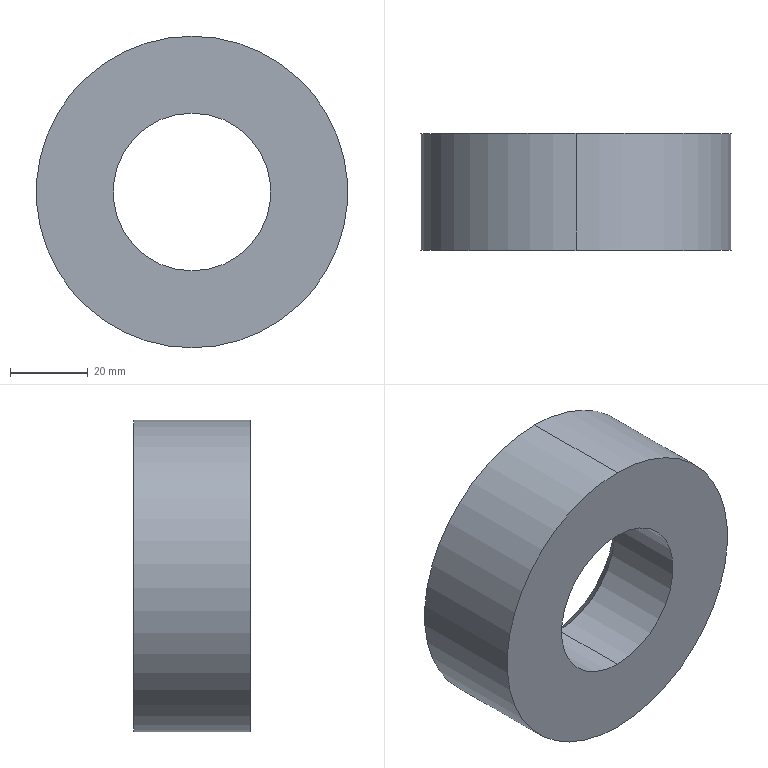Part | SolidWorks | features HoleWzd 1, Revolution 1 | 1 solid | 11 faces | box 80 x 30 x 80 mm | volume 100918 mm3 | cylinder 4 | cone 4 | plane 3 | commonest cylinder face diameters 40.5 x2 80 x2
STEP:
#1=CARTESIAN_POINT('',(0.,21.25,-20.25));
#2=VERTEX_POINT('',#1);
#3=CARTESIAN_POINT('',(0.,21.25,20.25));
#4=VERTEX_POINT('',#3);
#5=CARTESIAN_POINT('',(0.,21.25,0.));
#6=DIRECTION('',(0.,1.,0.));
#7=DIRECTION('',(0.,0.,1.));
#8=AXIS2_PLACEMENT_3D('',#5,#6,#7);
#9=CIRCLE('',#8,20.25);
#10=EDGE_CURVE('',#2,#4,#9,.T.);
#11=ORIENTED_EDGE('',*,*,#10,.T.);
#12=CARTESIAN_POINT('',(0.,0.,20.25));
#13=VERTEX_POINT('',#12);
#14=CARTESIAN_POINT('',(0.,0.,20.25));
#15=DIRECTION('',(0.,-1.,0.));
#16=VECTOR('',#15,1000.);
#17=LINE('',#14,#16);
#18=EDGE_CURVE('',#4,#13,#17,.T.);
#19=ORIENTED_EDGE('',*,*,#18,.T.);
#20=CARTESIAN_POINT('',(0.,0.,-20.25));
#21=VERTEX_POINT('',#20);
#22=CARTESIAN_POINT('',(0.,0.,0.));
#23=DIRECTION('',(0.,-1.,0.));
#24=DIRECTION('',(0.,0.,-1.));
#25=AXIS2_PLACEMENT_3D('',#22,#23,#24);
#26=CIRCLE('',#25,20.25);
#27=EDGE_CURVE('',#13,#21,#26,.T.);
#28=ORIENTED_EDGE('',*,*,#27,.T.);
#29=CARTESIAN_POINT('',(0.,0.,-20.25));
#30=DIRECTION('',(0.,-1.,0.));
#31=VECTOR('',#30,1000.);
#32=LINE('',#29,#31);
#33=EDGE_CURVE('',#2,#21,#32,.T.);
#34=ORIENTED_EDGE('',*,*,#33,.F.);
#35=EDGE_LOOP('',(#11,#19,#28,#34));
#36=FACE_OUTER_BOUND('',#35,.T.);
#37=CARTESIAN_POINT('',(0.,0.,0.));
#38=DIRECTION('',(0.,-1.,0.));
#39=DIRECTION('',(0.,0.,-1.));
#40=AXIS2_PLACEMENT_3D('',#37,#38,#39);
#41=CYLINDRICAL_SURFACE('',#40,20.25);
#42=ADVANCED_FACE('',(#36),#41,.F.);
#43=ORIENTED_EDGE('',*,*,#10,.F.);
#44=CARTESIAN_POINT('',(0.,25.,-24.));
#45=VERTEX_POINT('',#44);
#46=CARTESIAN_POINT('',(0.,25.,-24.));
#47=DIRECTION('',(0.,0.7071,-0.7071));
#48=VECTOR('',#47,1000.);
#49=LINE('',#46,#48);
#50=EDGE_CURVE('',#2,#45,#49,.T.);
#51=ORIENTED_EDGE('',*,*,#50,.T.);
#52=CARTESIAN_POINT('',(0.,25.,24.));
#53=VERTEX_POINT('',#52);
#54=CARTESIAN_POINT('',(0.,25.,0.));
#55=DIRECTION('',(0.,-1.,0.));
#56=DIRECTION('',(0.,0.,-1.));
#57=AXIS2_PLACEMENT_3D('',#54,#55,#56);
#58=CIRCLE('',#57,24.);
#59=EDGE_CURVE('',#53,#45,#58,.T.);
#60=ORIENTED_EDGE('',*,*,#59,.F.);
#61=CARTESIAN_POINT('',(0.,25.,24.));
#62=DIRECTION('',(0.,0.7071,0.7071));
#63=VECTOR('',#62,1000.);
#64=LINE('',#61,#63);
#65=EDGE_CURVE('',#4,#53,#64,.T.);
#66=ORIENTED_EDGE('',*,*,#65,.F.);
#67=EDGE_LOOP('',(#43,#51,#60,#66));
#68=FACE_OUTER_BOUND('',#67,.T.);
#69=CARTESIAN_POINT('',(0.,25.,0.));
#70=DIRECTION('',(0.,1.,0.));
#71=DIRECTION('',(0.,0.,1.));
#72=AXIS2_PLACEMENT_3D('',#69,#70,#71);
#73=CONICAL_SURFACE('',#72,24.,0.7854);
#74=ADVANCED_FACE('',(#68),#73,.F.);
#75=CARTESIAN_POINT('',(0.,25.,27.5));
#76=VERTEX_POINT('',#75);
#77=CARTESIAN_POINT('',(0.,25.,-27.5));
#78=VERTEX_POINT('',#77);
#79=CARTESIAN_POINT('',(0.,25.,0.));
#80=DIRECTION('',(0.,-1.,0.));
#81=DIRECTION('',(0.,0.,-1.));
#82=AXIS2_PLACEMENT_3D('',#79,#80,#81);
#83=CIRCLE('',#82,27.5);
#84=EDGE_CURVE('',#76,#78,#83,.T.);
#85=ORIENTED_EDGE('',*,*,#84,.T.);
#86=CARTESIAN_POINT('',(0.,30.,-37.5));
#87=VERTEX_POINT('',#86);
#88=CARTESIAN_POINT('',(0.,30.,-37.5));
#89=DIRECTION('',(0.,0.4472,-0.8944));
#90=VECTOR('',#89,1000.);
#91=LINE('',#88,#90);
#92=EDGE_CURVE('',#78,#87,#91,.T.);
#93=ORIENTED_EDGE('',*,*,#92,.T.);
#94=CARTESIAN_POINT('',(0.,30.,37.5));
#95=VERTEX_POINT('',#94);
#96=CARTESIAN_POINT('',(0.,30.,0.));
#97=DIRECTION('',(0.,-1.,0.));
#98=DIRECTION('',(0.,0.,-1.));
#99=AXIS2_PLACEMENT_3D('',#96,#97,#98);
#100=CIRCLE('',#99,37.5);
#101=EDGE_CURVE('',#95,#87,#100,.T.);
#102=ORIENTED_EDGE('',*,*,#101,.F.);
#103=CARTESIAN_POINT('',(0.,30.,37.5));
#104=DIRECTION('',(0.,0.4472,0.8944));
#105=VECTOR('',#104,1000.);
#106=LINE('',#103,#105);
#107=EDGE_CURVE('',#76,#95,#106,.T.);
#108=ORIENTED_EDGE('',*,*,#107,.F.);
#109=EDGE_LOOP('',(#85,#93,#102,#108));
#110=FACE_OUTER_BOUND('',#109,.T.);
#111=CARTESIAN_POINT('',(0.,30.,0.));
#112=DIRECTION('',(0.,1.,0.));
#113=DIRECTION('',(0.,0.,1.));
#114=AXIS2_PLACEMENT_3D('',#111,#112,#113);
#115=CONICAL_SURFACE('',#114,37.5,1.107);
#116=ADVANCED_FACE('',(#110),#115,.F.);
#117=CARTESIAN_POINT('',(0.,30.,-40.));
#118=VERTEX_POINT('',#117);
#119=CARTESIAN_POINT('',(0.,30.,40.));
#120=VERTEX_POINT('',#119);
#121=CARTESIAN_POINT('',(0.,30.,0.));
#122=DIRECTION('',(0.,-1.,0.));
#123=DIRECTION('',(0.,0.,-1.));
#124=AXIS2_PLACEMENT_3D('',#121,#122,#123);
#125=CIRCLE('',#124,40.);
#126=EDGE_CURVE('',#118,#120,#125,.T.);
#127=ORIENTED_EDGE('',*,*,#126,.T.);
#128=CARTESIAN_POINT('',(0.,0.,40.));
#129=VERTEX_POINT('',#128);
#130=CARTESIAN_POINT('',(0.,0.,40.));
#131=DIRECTION('',(0.,-1.,0.));
#132=VECTOR('',#131,1000.);
#133=LINE('',#130,#132);
#134=EDGE_CURVE('',#120,#129,#133,.T.);
#135=ORIENTED_EDGE('',*,*,#134,.T.);
#136=CARTESIAN_POINT('',(0.,0.,-40.));
#137=VERTEX_POINT('',#136);
#138=CARTESIAN_POINT('',(0.,0.,0.));
#139=DIRECTION('',(0.,-1.,0.));
#140=DIRECTION('',(0.,0.,-1.));
#141=AXIS2_PLACEMENT_3D('',#138,#139,#140);
#142=CIRCLE('',#141,40.);
#143=EDGE_CURVE('',#137,#129,#142,.T.);
#144=ORIENTED_EDGE('',*,*,#143,.F.);
#145=CARTESIAN_POINT('',(0.,0.,-40.));
#146=DIRECTION('',(0.,-1.,0.));
#147=VECTOR('',#146,1000.);
#148=LINE('',#145,#147);
#149=EDGE_CURVE('',#118,#137,#148,.T.);
#150=ORIENTED_EDGE('',*,*,#149,.F.);
#151=EDGE_LOOP('',(#127,#135,#144,#150));
#152=FACE_OUTER_BOUND('',#151,.T.);
#153=CARTESIAN_POINT('',(0.,0.,0.));
#154=DIRECTION('',(0.,-1.,0.));
#155=DIRECTION('',(0.,0.,-1.));
#156=AXIS2_PLACEMENT_3D('',#153,#154,#155);
#157=CYLINDRICAL_SURFACE('',#156,40.);
#158=ADVANCED_FACE('',(#152),#157,.T.);
#159=ORIENTED_EDGE('',*,*,#134,.F.);
#160=CARTESIAN_POINT('',(0.,30.,0.));
#161=DIRECTION('',(0.,-1.,0.));
#162=DIRECTION('',(0.,0.,-1.));
#163=AXIS2_PLACEMENT_3D('',#160,#161,#162);
#164=CIRCLE('',#163,40.);
#165=EDGE_CURVE('',#120,#118,#164,.T.);
#166=ORIENTED_EDGE('',*,*,#165,.T.);
#167=ORIENTED_EDGE('',*,*,#149,.T.);
#168=CARTESIAN_POINT('',(0.,0.,0.));
#169=DIRECTION('',(0.,-1.,0.));
#170=DIRECTION('',(0.,0.,-1.));
#171=AXIS2_PLACEMENT_3D('',#168,#169,#170);
#172=CIRCLE('',#171,40.);
#173=EDGE_CURVE('',#129,#137,#172,.T.);
#174=ORIENTED_EDGE('',*,*,#173,.F.);
#175=EDGE_LOOP('',(#159,#166,#167,#174));
#176=FACE_OUTER_BOUND('',#175,.T.);
#177=CARTESIAN_POINT('',(0.,0.,0.));
#178=DIRECTION('',(0.,-1.,0.));
#179=DIRECTION('',(0.,0.,-1.));
#180=AXIS2_PLACEMENT_3D('',#177,#178,#179);
#181=CYLINDRICAL_SURFACE('',#180,40.);
#182=ADVANCED_FACE('',(#176),#181,.T.);
#183=ORIENTED_EDGE('',*,*,#101,.T.);
#184=CARTESIAN_POINT('',(0.,30.,0.));
#185=DIRECTION('',(0.,-1.,0.));
#186=DIRECTION('',(0.,0.,-1.));
#187=AXIS2_PLACEMENT_3D('',#184,#185,#186);
#188=CIRCLE('',#187,37.5);
#189=EDGE_CURVE('',#87,#95,#188,.T.);
#190=ORIENTED_EDGE('',*,*,#189,.T.);
#191=EDGE_LOOP('',(#183,#190));
#192=FACE_BOUND('',#191,.T.);
#193=ORIENTED_EDGE('',*,*,#126,.F.);
#194=ORIENTED_EDGE('',*,*,#165,.F.);
#195=EDGE_LOOP('',(#193,#194));
#196=FACE_OUTER_BOUND('',#195,.T.);
#197=CARTESIAN_POINT('',(40.,30.,0.));
#198=DIRECTION('',(0.,1.,0.));
#199=DIRECTION('',(0.,0.,1.));
#200=AXIS2_PLACEMENT_3D('',#197,#198,#199);
#201=PLANE('',#200);
#202=ADVANCED_FACE('',(#192,#196),#201,.T.);
#203=ORIENTED_EDGE('',*,*,#92,.F.);
#204=CARTESIAN_POINT('',(0.,25.,0.));
#205=DIRECTION('',(0.,-1.,0.));
#206=DIRECTION('',(0.,0.,-1.));
#207=AXIS2_PLACEMENT_3D('',#204,#205,#206);
#208=CIRCLE('',#207,27.5);
#209=EDGE_CURVE('',#78,#76,#208,.T.);
#210=ORIENTED_EDGE('',*,*,#209,.T.);
#211=ORIENTED_EDGE('',*,*,#107,.T.);
#212=ORIENTED_EDGE('',*,*,#189,.F.);
#213=EDGE_LOOP('',(#203,#210,#211,#212));
#214=FACE_OUTER_BOUND('',#213,.T.);
#215=CARTESIAN_POINT('',(0.,30.,0.));
#216=DIRECTION('',(0.,1.,0.));
#217=DIRECTION('',(0.,0.,1.));
#218=AXIS2_PLACEMENT_3D('',#215,#216,#217);
#219=CONICAL_SURFACE('',#218,37.5,1.107);
#220=ADVANCED_FACE('',(#214),#219,.F.);
#221=ORIENTED_EDGE('',*,*,#59,.T.);
#222=CARTESIAN_POINT('',(0.,25.,0.));
#223=DIRECTION('',(0.,-1.,0.));
#224=DIRECTION('',(0.,0.,-1.));
#225=AXIS2_PLACEMENT_3D('',#222,#223,#224);
#226=CIRCLE('',#225,24.);
#227=EDGE_CURVE('',#45,#53,#226,.T.);
#228=ORIENTED_EDGE('',*,*,#227,.T.);
#229=EDGE_LOOP('',(#221,#228));
#230=FACE_BOUND('',#229,.T.);
#231=ORIENTED_EDGE('',*,*,#84,.F.);
#232=ORIENTED_EDGE('',*,*,#209,.F.);
#233=EDGE_LOOP('',(#231,#232));
#234=FACE_OUTER_BOUND('',#233,.T.);
#235=CARTESIAN_POINT('',(27.5,25.,0.));
#236=DIRECTION('',(0.,1.,0.));
#237=DIRECTION('',(0.,0.,1.));
#238=AXIS2_PLACEMENT_3D('',#235,#236,#237);
#239=PLANE('',#238);
#240=ADVANCED_FACE('',(#230,#234),#239,.T.);
#241=ORIENTED_EDGE('',*,*,#50,.F.);
#242=CARTESIAN_POINT('',(0.,21.25,0.));
#243=DIRECTION('',(0.,1.,0.));
#244=DIRECTION('',(0.,0.,1.));
#245=AXIS2_PLACEMENT_3D('',#242,#243,#244);
#246=CIRCLE('',#245,20.25);
#247=EDGE_CURVE('',#4,#2,#246,.T.);
#248=ORIENTED_EDGE('',*,*,#247,.F.);
#249=ORIENTED_EDGE('',*,*,#65,.T.);
#250=ORIENTED_EDGE('',*,*,#227,.F.);
#251=EDGE_LOOP('',(#241,#248,#249,#250));
#252=FACE_OUTER_BOUND('',#251,.T.);
#253=CARTESIAN_POINT('',(0.,25.,0.));
#254=DIRECTION('',(0.,1.,0.));
#255=DIRECTION('',(0.,0.,1.));
#256=AXIS2_PLACEMENT_3D('',#253,#254,#255);
#257=CONICAL_SURFACE('',#256,24.,0.7854);
#258=ADVANCED_FACE('',(#252),#257,.F.);
#259=CARTESIAN_POINT('',(0.,0.,0.));
#260=DIRECTION('',(0.,-1.,0.));
#261=DIRECTION('',(0.,0.,-1.));
#262=AXIS2_PLACEMENT_3D('',#259,#260,#261);
#263=CIRCLE('',#262,20.25);
#264=EDGE_CURVE('',#21,#13,#263,.T.);
#265=ORIENTED_EDGE('',*,*,#264,.F.);
#266=ORIENTED_EDGE('',*,*,#27,.F.);
#267=EDGE_LOOP('',(#265,#266));
#268=FACE_BOUND('',#267,.T.);
#269=ORIENTED_EDGE('',*,*,#143,.T.);
#270=ORIENTED_EDGE('',*,*,#173,.T.);
#271=EDGE_LOOP('',(#269,#270));
#272=FACE_OUTER_BOUND('',#271,.T.);
#273=CARTESIAN_POINT('',(20.,0.,0.));
#274=DIRECTION('',(0.,-1.,0.));
#275=DIRECTION('',(0.,0.,-1.));
#276=AXIS2_PLACEMENT_3D('',#273,#274,#275);
#277=PLANE('',#276);
#278=ADVANCED_FACE('',(#268,#272),#277,.T.);
#279=ORIENTED_EDGE('',*,*,#18,.F.);
#280=ORIENTED_EDGE('',*,*,#247,.T.);
#281=ORIENTED_EDGE('',*,*,#33,.T.);
#282=ORIENTED_EDGE('',*,*,#264,.T.);
#283=EDGE_LOOP('',(#279,#280,#281,#282));
#284=FACE_OUTER_BOUND('',#283,.T.);
#285=CARTESIAN_POINT('',(0.,0.,0.));
#286=DIRECTION('',(0.,-1.,0.));
#287=DIRECTION('',(0.,0.,-1.));
#288=AXIS2_PLACEMENT_3D('',#285,#286,#287);
#289=CYLINDRICAL_SURFACE('',#288,20.25);
#290=ADVANCED_FACE('',(#284),#289,.F.);
#291=CLOSED_SHELL('',(#42,#74,#116,#158,#182,#202,#220,#240,#258,#278,#290));
#292=MANIFOLD_SOLID_BREP('',#291);
#293=CARTESIAN_POINT('',(0.,0.,0.));
#294=DIRECTION('',(0.,0.,1.));
#295=DIRECTION('',(1.,0.,0.));
#296=AXIS2_PLACEMENT_3D('',#293,#294,#295);
#297=(LENGTH_UNIT()NAMED_UNIT(*)SI_UNIT(.MILLI.,.METRE.));
#298=UNCERTAINTY_MEASURE_WITH_UNIT(LENGTH_MEASURE(0.00001),#297,'','');
#299=(NAMED_UNIT(*)PLANE_ANGLE_UNIT()SI_UNIT($,.RADIAN.));
#300=(NAMED_UNIT(*)SI_UNIT($,.STERADIAN.)SOLID_ANGLE_UNIT());
#301=(GEOMETRIC_REPRESENTATION_CONTEXT(3)GLOBAL_UNCERTAINTY_ASSIGNED_CONTEXT((#298))GLOBAL_UNIT_ASSIGNED_CONTEXT((#297,#299,#300))REPRESENTATION_CONTEXT('',''));
#302=ADVANCED_BREP_SHAPE_REPRESENTATION('',(#292,#296),#301);